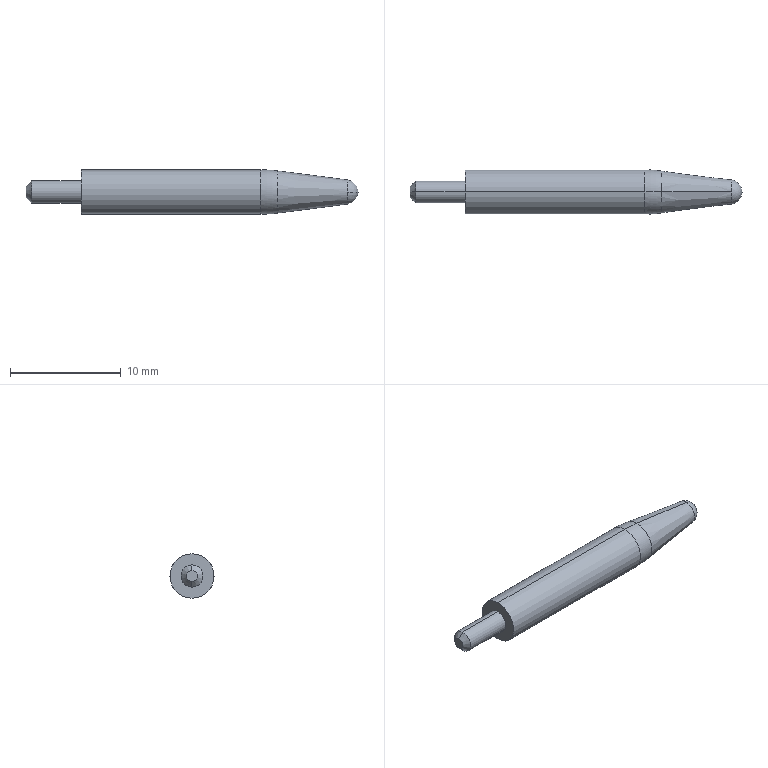Part | SolidWorks | features Chamfer 1, ICE 1, Revolution 1 | 1 solid | 14 faces | box 30 x 4 x 4 mm | volume 285.134 mm3 | cone 4 | cylinder 4 | plane 2 | torus 2 | sphere 2 | commonest cylinder face diameters 2 x2 4 x2
STEP:
#1=CARTESIAN_POINT('',(-5.,0.,0.5));
#2=VERTEX_POINT('',#1);
#3=CARTESIAN_POINT('',(-5.,0.,-0.5));
#4=VERTEX_POINT('',#3);
#5=CARTESIAN_POINT('',(-5.,0.,0.));
#6=DIRECTION('',(-1.,0.,0.));
#7=DIRECTION('',(0.,0.,1.));
#8=AXIS2_PLACEMENT_3D('',#5,#6,#7);
#9=CIRCLE('',#8,0.5);
#10=EDGE_CURVE('',#2,#4,#9,.T.);
#11=ORIENTED_EDGE('',*,*,#10,.F.);
#12=CARTESIAN_POINT('',(-4.5,0.,1.));
#13=VERTEX_POINT('',#12);
#14=CARTESIAN_POINT('',(-5.,0.,0.5));
#15=DIRECTION('',(0.7071,0.,0.7071));
#16=VECTOR('',#15,1000.);
#17=LINE('',#14,#16);
#18=EDGE_CURVE('',#2,#13,#17,.T.);
#19=ORIENTED_EDGE('',*,*,#18,.T.);
#20=CARTESIAN_POINT('',(-4.5,0.,-1.));
#21=VERTEX_POINT('',#20);
#22=CARTESIAN_POINT('',(-4.5,0.,0.));
#23=DIRECTION('',(1.,0.,0.));
#24=DIRECTION('',(0.,0.,1.));
#25=AXIS2_PLACEMENT_3D('',#22,#23,#24);
#26=CIRCLE('',#25,1.);
#27=EDGE_CURVE('',#21,#13,#26,.T.);
#28=ORIENTED_EDGE('',*,*,#27,.F.);
#29=CARTESIAN_POINT('',(-5.,0.,-0.5));
#30=DIRECTION('',(0.7071,0.,-0.7071));
#31=VECTOR('',#30,1000.);
#32=LINE('',#29,#31);
#33=EDGE_CURVE('',#4,#21,#32,.T.);
#34=ORIENTED_EDGE('',*,*,#33,.F.);
#35=EDGE_LOOP('',(#11,#19,#28,#34));
#36=FACE_OUTER_BOUND('',#35,.T.);
#37=CARTESIAN_POINT('',(-5.,0.,0.));
#38=DIRECTION('',(1.,0.,0.));
#39=DIRECTION('',(0.,0.,-1.));
#40=AXIS2_PLACEMENT_3D('',#37,#38,#39);
#41=CONICAL_SURFACE('',#40,0.5,0.7854);
#42=ADVANCED_FACE('',(#36),#41,.T.);
#43=ORIENTED_EDGE('',*,*,#27,.T.);
#44=CARTESIAN_POINT('',(0.,0.,1.));
#45=VERTEX_POINT('',#44);
#46=CARTESIAN_POINT('',(-5.,0.,1.));
#47=DIRECTION('',(1.,0.,0.));
#48=VECTOR('',#47,1000.);
#49=LINE('',#46,#48);
#50=EDGE_CURVE('',#13,#45,#49,.T.);
#51=ORIENTED_EDGE('',*,*,#50,.T.);
#52=CARTESIAN_POINT('',(0.,0.,-1.));
#53=VERTEX_POINT('',#52);
#54=CARTESIAN_POINT('',(0.,0.,0.));
#55=DIRECTION('',(-1.,0.,0.));
#56=DIRECTION('',(0.,0.,1.));
#57=AXIS2_PLACEMENT_3D('',#54,#55,#56);
#58=CIRCLE('',#57,1.);
#59=EDGE_CURVE('',#45,#53,#58,.T.);
#60=ORIENTED_EDGE('',*,*,#59,.T.);
#61=CARTESIAN_POINT('',(-5.,0.,-1.));
#62=DIRECTION('',(1.,0.,0.));
#63=VECTOR('',#62,1000.);
#64=LINE('',#61,#63);
#65=EDGE_CURVE('',#21,#53,#64,.T.);
#66=ORIENTED_EDGE('',*,*,#65,.F.);
#67=EDGE_LOOP('',(#43,#51,#60,#66));
#68=FACE_OUTER_BOUND('',#67,.T.);
#69=CARTESIAN_POINT('',(-5.,0.,0.));
#70=DIRECTION('',(1.,0.,0.));
#71=DIRECTION('',(0.,0.,-1.));
#72=AXIS2_PLACEMENT_3D('',#69,#70,#71);
#73=CYLINDRICAL_SURFACE('',#72,1.);
#74=ADVANCED_FACE('',(#68),#73,.T.);
#75=CARTESIAN_POINT('',(16.229,0.,2.));
#76=VERTEX_POINT('',#75);
#77=CARTESIAN_POINT('',(16.229,0.,-2.));
#78=VERTEX_POINT('',#77);
#79=CARTESIAN_POINT('',(16.229,0.,0.));
#80=DIRECTION('',(-1.,0.,0.));
#81=DIRECTION('',(0.,0.,1.));
#82=AXIS2_PLACEMENT_3D('',#79,#80,#81);
#83=CIRCLE('',#82,2.);
#84=EDGE_CURVE('',#76,#78,#83,.T.);
#85=ORIENTED_EDGE('',*,*,#84,.T.);
#86=CARTESIAN_POINT('',(0.,0.,-2.));
#87=VERTEX_POINT('',#86);
#88=CARTESIAN_POINT('',(0.,0.,-2.));
#89=DIRECTION('',(-1.,0.,0.));
#90=VECTOR('',#89,1000.);
#91=LINE('',#88,#90);
#92=EDGE_CURVE('',#78,#87,#91,.T.);
#93=ORIENTED_EDGE('',*,*,#92,.T.);
#94=CARTESIAN_POINT('',(0.,0.,2.));
#95=VERTEX_POINT('',#94);
#96=CARTESIAN_POINT('',(0.,0.,0.));
#97=DIRECTION('',(-1.,0.,0.));
#98=DIRECTION('',(0.,0.,1.));
#99=AXIS2_PLACEMENT_3D('',#96,#97,#98);
#100=CIRCLE('',#99,2.);
#101=EDGE_CURVE('',#95,#87,#100,.T.);
#102=ORIENTED_EDGE('',*,*,#101,.F.);
#103=CARTESIAN_POINT('',(0.,0.,2.));
#104=DIRECTION('',(-1.,0.,0.));
#105=VECTOR('',#104,1000.);
#106=LINE('',#103,#105);
#107=EDGE_CURVE('',#76,#95,#106,.T.);
#108=ORIENTED_EDGE('',*,*,#107,.F.);
#109=EDGE_LOOP('',(#85,#93,#102,#108));
#110=FACE_OUTER_BOUND('',#109,.T.);
#111=CARTESIAN_POINT('',(0.,0.,0.));
#112=DIRECTION('',(-1.,0.,0.));
#113=DIRECTION('',(0.,0.,1.));
#114=AXIS2_PLACEMENT_3D('',#111,#112,#113);
#115=CYLINDRICAL_SURFACE('',#114,2.);
#116=ADVANCED_FACE('',(#110),#115,.T.);
#117=CARTESIAN_POINT('',(17.765,0.,1.901));
#118=VERTEX_POINT('',#117);
#119=CARTESIAN_POINT('',(17.765,0.,-1.901));
#120=VERTEX_POINT('',#119);
#121=CARTESIAN_POINT('',(17.765,0.,0.));
#122=DIRECTION('',(-1.,0.,0.));
#123=DIRECTION('',(0.,0.,1.));
#124=AXIS2_PLACEMENT_3D('',#121,#122,#123);
#125=CIRCLE('',#124,1.901);
#126=EDGE_CURVE('',#118,#120,#125,.T.);
#127=ORIENTED_EDGE('',*,*,#126,.T.);
#128=CARTESIAN_POINT('',(16.229,0.,10.));
#129=DIRECTION('',(0.,1.,0.));
#130=DIRECTION('',(0.,0.,1.));
#131=AXIS2_PLACEMENT_3D('',#128,#129,#130);
#132=CIRCLE('',#131,12.);
#133=EDGE_CURVE('',#120,#78,#132,.T.);
#134=ORIENTED_EDGE('',*,*,#133,.T.);
#135=ORIENTED_EDGE('',*,*,#84,.F.);
#136=CARTESIAN_POINT('',(16.229,0.,-10.));
#137=DIRECTION('',(0.,-1.,0.));
#138=DIRECTION('',(0.,0.,-1.));
#139=AXIS2_PLACEMENT_3D('',#136,#137,#138);
#140=CIRCLE('',#139,12.);
#141=EDGE_CURVE('',#118,#76,#140,.T.);
#142=ORIENTED_EDGE('',*,*,#141,.F.);
#143=EDGE_LOOP('',(#127,#134,#135,#142));
#144=FACE_OUTER_BOUND('',#143,.T.);
#145=CARTESIAN_POINT('',(16.229,0.,0.));
#146=DIRECTION('',(-1.,0.,0.));
#147=DIRECTION('',(0.,0.,1.));
#148=AXIS2_PLACEMENT_3D('',#145,#146,#147);
#149=TOROIDAL_SURFACE('',#148,-10.,12.);
#150=ADVANCED_FACE('',(#144),#149,.T.);
#151=CARTESIAN_POINT('',(24.041,1.091,0.));
#152=VERTEX_POINT('',#151);
#153=CARTESIAN_POINT('',(24.041,0.,-1.091));
#154=VERTEX_POINT('',#153);
#155=CARTESIAN_POINT('',(24.041,0.,0.));
#156=DIRECTION('',(-1.,0.,0.));
#157=DIRECTION('',(0.,0.,1.));
#158=AXIS2_PLACEMENT_3D('',#155,#156,#157);
#159=CIRCLE('',#158,1.091);
#160=EDGE_CURVE('',#152,#154,#159,.T.);
#161=ORIENTED_EDGE('',*,*,#160,.T.);
#162=CARTESIAN_POINT('',(24.041,0.,-1.091));
#163=DIRECTION('',(-0.9918,0.,-0.128));
#164=VECTOR('',#163,1000.);
#165=LINE('',#162,#164);
#166=EDGE_CURVE('',#154,#120,#165,.T.);
#167=ORIENTED_EDGE('',*,*,#166,.T.);
#168=ORIENTED_EDGE('',*,*,#126,.F.);
#169=CARTESIAN_POINT('',(24.041,0.,1.091));
#170=VERTEX_POINT('',#169);
#171=CARTESIAN_POINT('',(24.041,0.,1.091));
#172=DIRECTION('',(-0.9918,0.,0.128));
#173=VECTOR('',#172,1000.);
#174=LINE('',#171,#173);
#175=EDGE_CURVE('',#170,#118,#174,.T.);
#176=ORIENTED_EDGE('',*,*,#175,.F.);
#177=CARTESIAN_POINT('',(24.041,0.,0.));
#178=DIRECTION('',(-1.,0.,0.));
#179=DIRECTION('',(0.,0.,1.));
#180=AXIS2_PLACEMENT_3D('',#177,#178,#179);
#181=CIRCLE('',#180,1.091);
#182=EDGE_CURVE('',#170,#152,#181,.T.);
#183=ORIENTED_EDGE('',*,*,#182,.T.);
#184=EDGE_LOOP('',(#161,#167,#168,#176,#183));
#185=FACE_OUTER_BOUND('',#184,.T.);
#186=CARTESIAN_POINT('',(24.041,0.,0.));
#187=DIRECTION('',(-1.,0.,0.));
#188=DIRECTION('',(0.,0.,1.));
#189=AXIS2_PLACEMENT_3D('',#186,#187,#188);
#190=CONICAL_SURFACE('',#189,1.091,0.1284);
#191=ADVANCED_FACE('',(#185),#190,.T.);
#192=CARTESIAN_POINT('',(25.,0.,0.));
#193=VERTEX_POINT('',#192);
#194=CARTESIAN_POINT('',(23.9,0.,0.));
#195=DIRECTION('',(0.,0.,1.));
#196=DIRECTION('',(1.,0.,0.));
#197=AXIS2_PLACEMENT_3D('',#194,#195,#196);
#198=CIRCLE('',#197,1.1);
#199=EDGE_CURVE('',#193,#152,#198,.T.);
#200=ORIENTED_EDGE('',*,*,#199,.F.);
#201=CARTESIAN_POINT('',(24.041,-1.091,0.));
#202=VERTEX_POINT('',#201);
#203=CARTESIAN_POINT('',(23.9,0.,0.));
#204=DIRECTION('',(0.,0.,-1.));
#205=DIRECTION('',(0.,1.,0.));
#206=AXIS2_PLACEMENT_3D('',#203,#204,#205);
#207=CIRCLE('',#206,1.1);
#208=EDGE_CURVE('',#193,#202,#207,.T.);
#209=ORIENTED_EDGE('',*,*,#208,.T.);
#210=CARTESIAN_POINT('',(24.041,0.,0.));
#211=DIRECTION('',(-1.,0.,0.));
#212=DIRECTION('',(0.,0.,1.));
#213=AXIS2_PLACEMENT_3D('',#210,#211,#212);
#214=CIRCLE('',#213,1.091);
#215=EDGE_CURVE('',#154,#202,#214,.T.);
#216=ORIENTED_EDGE('',*,*,#215,.F.);
#217=ORIENTED_EDGE('',*,*,#160,.F.);
#218=EDGE_LOOP('',(#200,#209,#216,#217));
#219=FACE_OUTER_BOUND('',#218,.T.);
#220=CARTESIAN_POINT('',(23.9,0.,0.));
#221=DIRECTION('',(0.,0.,-1.));
#222=DIRECTION('',(0.,1.,0.));
#223=AXIS2_PLACEMENT_3D('',#220,#221,#222);
#224=SPHERICAL_SURFACE('',#223,1.1);
#225=ADVANCED_FACE('',(#219),#224,.T.);
#226=ORIENTED_EDGE('',*,*,#208,.F.);
#227=ORIENTED_EDGE('',*,*,#199,.T.);
#228=ORIENTED_EDGE('',*,*,#182,.F.);
#229=CARTESIAN_POINT('',(24.041,0.,0.));
#230=DIRECTION('',(-1.,0.,0.));
#231=DIRECTION('',(0.,0.,1.));
#232=AXIS2_PLACEMENT_3D('',#229,#230,#231);
#233=CIRCLE('',#232,1.091);
#234=EDGE_CURVE('',#202,#170,#233,.T.);
#235=ORIENTED_EDGE('',*,*,#234,.F.);
#236=EDGE_LOOP('',(#226,#227,#228,#235));
#237=FACE_OUTER_BOUND('',#236,.T.);
#238=CARTESIAN_POINT('',(23.9,0.,0.));
#239=DIRECTION('',(0.,0.,-1.));
#240=DIRECTION('',(0.,1.,0.));
#241=AXIS2_PLACEMENT_3D('',#238,#239,#240);
#242=SPHERICAL_SURFACE('',#241,1.1);
#243=ADVANCED_FACE('',(#237),#242,.T.);
#244=ORIENTED_EDGE('',*,*,#166,.F.);
#245=ORIENTED_EDGE('',*,*,#215,.T.);
#246=ORIENTED_EDGE('',*,*,#234,.T.);
#247=ORIENTED_EDGE('',*,*,#175,.T.);
#248=CARTESIAN_POINT('',(17.765,0.,0.));
#249=DIRECTION('',(-1.,0.,0.));
#250=DIRECTION('',(0.,0.,1.));
#251=AXIS2_PLACEMENT_3D('',#248,#249,#250);
#252=CIRCLE('',#251,1.901);
#253=EDGE_CURVE('',#120,#118,#252,.T.);
#254=ORIENTED_EDGE('',*,*,#253,.F.);
#255=EDGE_LOOP('',(#244,#245,#246,#247,#254));
#256=FACE_OUTER_BOUND('',#255,.T.);
#257=CARTESIAN_POINT('',(24.041,0.,0.));
#258=DIRECTION('',(-1.,0.,0.));
#259=DIRECTION('',(0.,0.,1.));
#260=AXIS2_PLACEMENT_3D('',#257,#258,#259);
#261=CONICAL_SURFACE('',#260,1.091,0.1284);
#262=ADVANCED_FACE('',(#256),#261,.T.);
#263=ORIENTED_EDGE('',*,*,#133,.F.);
#264=ORIENTED_EDGE('',*,*,#253,.T.);
#265=ORIENTED_EDGE('',*,*,#141,.T.);
#266=CARTESIAN_POINT('',(16.229,0.,0.));
#267=DIRECTION('',(-1.,0.,0.));
#268=DIRECTION('',(0.,0.,1.));
#269=AXIS2_PLACEMENT_3D('',#266,#267,#268);
#270=CIRCLE('',#269,2.);
#271=EDGE_CURVE('',#78,#76,#270,.T.);
#272=ORIENTED_EDGE('',*,*,#271,.F.);
#273=EDGE_LOOP('',(#263,#264,#265,#272));
#274=FACE_OUTER_BOUND('',#273,.T.);
#275=CARTESIAN_POINT('',(16.229,0.,0.));
#276=DIRECTION('',(-1.,0.,0.));
#277=DIRECTION('',(0.,0.,1.));
#278=AXIS2_PLACEMENT_3D('',#275,#276,#277);
#279=TOROIDAL_SURFACE('',#278,-10.,12.);
#280=ADVANCED_FACE('',(#274),#279,.T.);
#281=ORIENTED_EDGE('',*,*,#92,.F.);
#282=ORIENTED_EDGE('',*,*,#271,.T.);
#283=ORIENTED_EDGE('',*,*,#107,.T.);
#284=CARTESIAN_POINT('',(0.,0.,0.));
#285=DIRECTION('',(-1.,0.,0.));
#286=DIRECTION('',(0.,0.,1.));
#287=AXIS2_PLACEMENT_3D('',#284,#285,#286);
#288=CIRCLE('',#287,2.);
#289=EDGE_CURVE('',#87,#95,#288,.T.);
#290=ORIENTED_EDGE('',*,*,#289,.F.);
#291=EDGE_LOOP('',(#281,#282,#283,#290));
#292=FACE_OUTER_BOUND('',#291,.T.);
#293=CARTESIAN_POINT('',(0.,0.,0.));
#294=DIRECTION('',(-1.,0.,0.));
#295=DIRECTION('',(0.,0.,1.));
#296=AXIS2_PLACEMENT_3D('',#293,#294,#295);
#297=CYLINDRICAL_SURFACE('',#296,2.);
#298=ADVANCED_FACE('',(#292),#297,.T.);
#299=CARTESIAN_POINT('',(0.,0.,0.));
#300=DIRECTION('',(-1.,0.,0.));
#301=DIRECTION('',(0.,0.,1.));
#302=AXIS2_PLACEMENT_3D('',#299,#300,#301);
#303=CIRCLE('',#302,1.);
#304=EDGE_CURVE('',#53,#45,#303,.T.);
#305=ORIENTED_EDGE('',*,*,#304,.F.);
#306=ORIENTED_EDGE('',*,*,#59,.F.);
#307=EDGE_LOOP('',(#305,#306));
#308=FACE_BOUND('',#307,.T.);
#309=ORIENTED_EDGE('',*,*,#101,.T.);
#310=ORIENTED_EDGE('',*,*,#289,.T.);
#311=EDGE_LOOP('',(#309,#310));
#312=FACE_OUTER_BOUND('',#311,.T.);
#313=CARTESIAN_POINT('',(0.,0.,0.));
#314=DIRECTION('',(1.,0.,0.));
#315=DIRECTION('',(0.,0.,-1.));
#316=AXIS2_PLACEMENT_3D('',#313,#314,#315);
#317=PLANE('',#316);
#318=ADVANCED_FACE('',(#308,#312),#317,.F.);
#319=ORIENTED_EDGE('',*,*,#50,.F.);
#320=CARTESIAN_POINT('',(-4.5,0.,0.));
#321=DIRECTION('',(1.,0.,0.));
#322=DIRECTION('',(0.,0.,1.));
#323=AXIS2_PLACEMENT_3D('',#320,#321,#322);
#324=CIRCLE('',#323,1.);
#325=EDGE_CURVE('',#13,#21,#324,.T.);
#326=ORIENTED_EDGE('',*,*,#325,.T.);
#327=ORIENTED_EDGE('',*,*,#65,.T.);
#328=ORIENTED_EDGE('',*,*,#304,.T.);
#329=EDGE_LOOP('',(#319,#326,#327,#328));
#330=FACE_OUTER_BOUND('',#329,.T.);
#331=CARTESIAN_POINT('',(-5.,0.,0.));
#332=DIRECTION('',(1.,0.,0.));
#333=DIRECTION('',(0.,0.,-1.));
#334=AXIS2_PLACEMENT_3D('',#331,#332,#333);
#335=CYLINDRICAL_SURFACE('',#334,1.);
#336=ADVANCED_FACE('',(#330),#335,.T.);
#337=CARTESIAN_POINT('',(-5.,0.,0.));
#338=DIRECTION('',(-1.,0.,0.));
#339=DIRECTION('',(0.,0.,1.));
#340=AXIS2_PLACEMENT_3D('',#337,#338,#339);
#341=CIRCLE('',#340,0.5);
#342=EDGE_CURVE('',#4,#2,#341,.T.);
#343=ORIENTED_EDGE('',*,*,#342,.T.);
#344=ORIENTED_EDGE('',*,*,#10,.T.);
#345=EDGE_LOOP('',(#343,#344));
#346=FACE_OUTER_BOUND('',#345,.T.);
#347=CARTESIAN_POINT('',(-5.,0.,0.));
#348=DIRECTION('',(-1.,0.,0.));
#349=DIRECTION('',(0.,0.,1.));
#350=AXIS2_PLACEMENT_3D('',#347,#348,#349);
#351=PLANE('',#350);
#352=ADVANCED_FACE('',(#346),#351,.T.);
#353=ORIENTED_EDGE('',*,*,#18,.F.);
#354=ORIENTED_EDGE('',*,*,#342,.F.);
#355=ORIENTED_EDGE('',*,*,#33,.T.);
#356=ORIENTED_EDGE('',*,*,#325,.F.);
#357=EDGE_LOOP('',(#353,#354,#355,#356));
#358=FACE_OUTER_BOUND('',#357,.T.);
#359=CARTESIAN_POINT('',(-5.,0.,0.));
#360=DIRECTION('',(1.,0.,0.));
#361=DIRECTION('',(0.,0.,-1.));
#362=AXIS2_PLACEMENT_3D('',#359,#360,#361);
#363=CONICAL_SURFACE('',#362,0.5,0.7854);
#364=ADVANCED_FACE('',(#358),#363,.T.);
#365=CLOSED_SHELL('',(#42,#74,#116,#150,#191,#225,#243,#262,#280,#298,#318,#336,#352,#364));
#366=MANIFOLD_SOLID_BREP('',#365);
#367=CARTESIAN_POINT('',(0.,0.,0.));
#368=DIRECTION('',(0.,0.,1.));
#369=DIRECTION('',(1.,0.,0.));
#370=AXIS2_PLACEMENT_3D('',#367,#368,#369);
#371=(LENGTH_UNIT()NAMED_UNIT(*)SI_UNIT(.MILLI.,.METRE.));
#372=UNCERTAINTY_MEASURE_WITH_UNIT(LENGTH_MEASURE(0.00001),#371,'','');
#373=(NAMED_UNIT(*)PLANE_ANGLE_UNIT()SI_UNIT($,.RADIAN.));
#374=(NAMED_UNIT(*)SI_UNIT($,.STERADIAN.)SOLID_ANGLE_UNIT());
#375=(GEOMETRIC_REPRESENTATION_CONTEXT(3)GLOBAL_UNCERTAINTY_ASSIGNED_CONTEXT((#372))GLOBAL_UNIT_ASSIGNED_CONTEXT((#371,#373,#374))REPRESENTATION_CONTEXT('',''));
#376=ADVANCED_BREP_SHAPE_REPRESENTATION('',(#366,#370),#375);